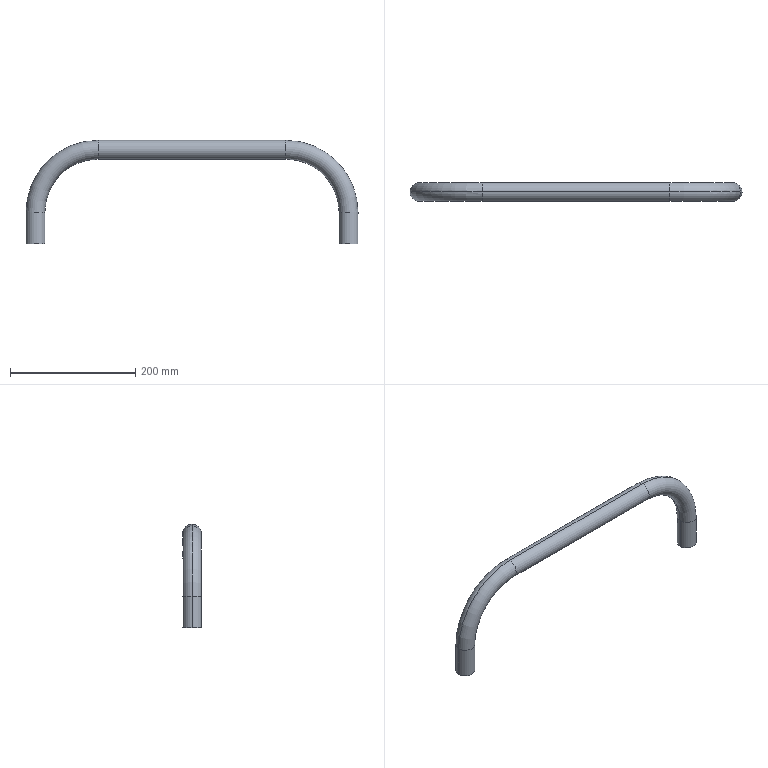Part | SolidWorks | features HoleWzd 1, Sweep 1 | 1 solid | 20 faces | box 530 x 30 x 165 mm | volume 501138 mm3 | cylinder 10 | torus 4 | cone 4 | plane 2 | commonest cylinder face diameters 30 x6 8.5 x4
STEP:
#1=CARTESIAN_POINT('',(400.,0.,15.));
#2=VERTEX_POINT('',#1);
#3=CARTESIAN_POINT('',(400.,0.,-15.));
#4=VERTEX_POINT('',#3);
#5=CARTESIAN_POINT('',(400.,0.,0.));
#6=DIRECTION('',(-1.,0.,0.));
#7=DIRECTION('',(0.,0.,1.));
#8=AXIS2_PLACEMENT_3D('',#5,#6,#7);
#9=CIRCLE('',#8,15.);
#10=EDGE_CURVE('',#2,#4,#9,.T.);
#11=ORIENTED_EDGE('',*,*,#10,.F.);
#12=CARTESIAN_POINT('',(515.,0.,-100.));
#13=VERTEX_POINT('',#12);
#14=CARTESIAN_POINT('',(400.,0.,-100.));
#15=DIRECTION('',(0.,1.,0.));
#16=DIRECTION('',(0.,0.,1.));
#17=AXIS2_PLACEMENT_3D('',#14,#15,#16);
#18=CIRCLE('',#17,115.);
#19=EDGE_CURVE('',#2,#13,#18,.T.);
#20=ORIENTED_EDGE('',*,*,#19,.T.);
#21=CARTESIAN_POINT('',(485.,0.,-100.));
#22=VERTEX_POINT('',#21);
#23=CARTESIAN_POINT('',(500.,0.,-100.));
#24=DIRECTION('',(0.,0.,1.));
#25=DIRECTION('',(1.,0.,0.));
#26=AXIS2_PLACEMENT_3D('',#23,#24,#25);
#27=CIRCLE('',#26,15.);
#28=EDGE_CURVE('',#13,#22,#27,.T.);
#29=ORIENTED_EDGE('',*,*,#28,.T.);
#30=CARTESIAN_POINT('',(400.,0.,-100.));
#31=DIRECTION('',(0.,1.,0.));
#32=DIRECTION('',(0.,0.,1.));
#33=AXIS2_PLACEMENT_3D('',#30,#31,#32);
#34=CIRCLE('',#33,85.);
#35=EDGE_CURVE('',#4,#22,#34,.T.);
#36=ORIENTED_EDGE('',*,*,#35,.F.);
#37=EDGE_LOOP('',(#11,#20,#29,#36));
#38=FACE_OUTER_BOUND('',#37,.T.);
#39=CARTESIAN_POINT('',(400.,0.,-100.));
#40=DIRECTION('',(0.,1.,0.));
#41=DIRECTION('',(0.,0.,1.));
#42=AXIS2_PLACEMENT_3D('',#39,#40,#41);
#43=TOROIDAL_SURFACE('',#42,100.,15.);
#44=ADVANCED_FACE('',(#38),#43,.T.);
#45=CARTESIAN_POINT('',(-15.,0.,-100.));
#46=VERTEX_POINT('',#45);
#47=CARTESIAN_POINT('',(15.,0.,-100.));
#48=VERTEX_POINT('',#47);
#49=CARTESIAN_POINT('',(0.,0.,-100.));
#50=DIRECTION('',(0.,0.,-1.));
#51=DIRECTION('',(-1.,0.,0.));
#52=AXIS2_PLACEMENT_3D('',#49,#50,#51);
#53=CIRCLE('',#52,15.);
#54=EDGE_CURVE('',#46,#48,#53,.T.);
#55=ORIENTED_EDGE('',*,*,#54,.F.);
#56=CARTESIAN_POINT('',(100.,0.,15.));
#57=VERTEX_POINT('',#56);
#58=CARTESIAN_POINT('',(100.,0.,-100.));
#59=DIRECTION('',(0.,1.,0.));
#60=DIRECTION('',(0.,0.,1.));
#61=AXIS2_PLACEMENT_3D('',#58,#59,#60);
#62=CIRCLE('',#61,115.);
#63=EDGE_CURVE('',#46,#57,#62,.T.);
#64=ORIENTED_EDGE('',*,*,#63,.T.);
#65=CARTESIAN_POINT('',(100.,0.,-15.));
#66=VERTEX_POINT('',#65);
#67=CARTESIAN_POINT('',(100.,0.,0.));
#68=DIRECTION('',(-1.,0.,0.));
#69=DIRECTION('',(0.,0.,1.));
#70=AXIS2_PLACEMENT_3D('',#67,#68,#69);
#71=CIRCLE('',#70,15.);
#72=EDGE_CURVE('',#57,#66,#71,.T.);
#73=ORIENTED_EDGE('',*,*,#72,.T.);
#74=CARTESIAN_POINT('',(100.,0.,-100.));
#75=DIRECTION('',(0.,1.,0.));
#76=DIRECTION('',(0.,0.,1.));
#77=AXIS2_PLACEMENT_3D('',#74,#75,#76);
#78=CIRCLE('',#77,85.);
#79=EDGE_CURVE('',#48,#66,#78,.T.);
#80=ORIENTED_EDGE('',*,*,#79,.F.);
#81=EDGE_LOOP('',(#55,#64,#73,#80));
#82=FACE_OUTER_BOUND('',#81,.T.);
#83=CARTESIAN_POINT('',(100.,0.,-100.));
#84=DIRECTION('',(0.,1.,0.));
#85=DIRECTION('',(0.,0.,1.));
#86=AXIS2_PLACEMENT_3D('',#83,#84,#85);
#87=TOROIDAL_SURFACE('',#86,100.,15.);
#88=ADVANCED_FACE('',(#82),#87,.T.);
#89=CARTESIAN_POINT('',(504.25,0.,-118.5));
#90=VERTEX_POINT('',#89);
#91=CARTESIAN_POINT('',(495.75,0.,-118.5));
#92=VERTEX_POINT('',#91);
#93=CARTESIAN_POINT('',(500.,0.,-118.5));
#94=DIRECTION('',(0.,0.,-1.));
#95=DIRECTION('',(-1.,0.,0.));
#96=AXIS2_PLACEMENT_3D('',#93,#94,#95);
#97=CIRCLE('',#96,4.25);
#98=EDGE_CURVE('',#90,#92,#97,.T.);
#99=ORIENTED_EDGE('',*,*,#98,.F.);
#100=CARTESIAN_POINT('',(504.25,0.,-150.));
#101=VERTEX_POINT('',#100);
#102=CARTESIAN_POINT('',(504.25,0.,-150.));
#103=DIRECTION('',(0.,0.,-1.));
#104=VECTOR('',#103,1000.);
#105=LINE('',#102,#104);
#106=EDGE_CURVE('',#90,#101,#105,.T.);
#107=ORIENTED_EDGE('',*,*,#106,.T.);
#108=CARTESIAN_POINT('',(495.75,0.,-150.));
#109=VERTEX_POINT('',#108);
#110=CARTESIAN_POINT('',(500.,0.,-150.));
#111=DIRECTION('',(0.,0.,-1.));
#112=DIRECTION('',(-1.,0.,0.));
#113=AXIS2_PLACEMENT_3D('',#110,#111,#112);
#114=CIRCLE('',#113,4.25);
#115=EDGE_CURVE('',#101,#109,#114,.T.);
#116=ORIENTED_EDGE('',*,*,#115,.T.);
#117=CARTESIAN_POINT('',(495.75,0.,-150.));
#118=DIRECTION('',(0.,0.,-1.));
#119=VECTOR('',#118,1000.);
#120=LINE('',#117,#119);
#121=EDGE_CURVE('',#92,#109,#120,.T.);
#122=ORIENTED_EDGE('',*,*,#121,.F.);
#123=EDGE_LOOP('',(#99,#107,#116,#122));
#124=FACE_OUTER_BOUND('',#123,.T.);
#125=CARTESIAN_POINT('',(500.,0.,-150.));
#126=DIRECTION('',(0.,0.,-1.));
#127=DIRECTION('',(-1.,0.,0.));
#128=AXIS2_PLACEMENT_3D('',#125,#126,#127);
#129=CYLINDRICAL_SURFACE('',#128,4.25);
#130=ADVANCED_FACE('',(#124),#129,.F.);
#131=CARTESIAN_POINT('',(500.,0.,-115.946));
#132=VERTEX_POINT('',#131);
#133=CARTESIAN_POINT('',(495.75,0.,-118.5));
#134=DIRECTION('',(-0.8572,0.,-0.515));
#135=VECTOR('',#134,1000.);
#136=LINE('',#133,#135);
#137=EDGE_CURVE('',#132,#92,#136,.T.);
#138=ORIENTED_EDGE('',*,*,#137,.F.);
#139=CARTESIAN_POINT('',(504.25,0.,-118.5));
#140=DIRECTION('',(0.8572,0.,-0.515));
#141=VECTOR('',#140,1000.);
#142=LINE('',#139,#141);
#143=EDGE_CURVE('',#132,#90,#142,.T.);
#144=ORIENTED_EDGE('',*,*,#143,.T.);
#145=ORIENTED_EDGE('',*,*,#98,.T.);
#146=EDGE_LOOP('',(#138,#144,#145));
#147=FACE_OUTER_BOUND('',#146,.T.);
#148=CARTESIAN_POINT('',(500.,0.,-118.5));
#149=DIRECTION('',(0.,0.,-1.));
#150=DIRECTION('',(-1.,0.,0.));
#151=AXIS2_PLACEMENT_3D('',#148,#149,#150);
#152=CONICAL_SURFACE('',#151,4.25,1.03);
#153=ADVANCED_FACE('',(#147),#152,.F.);
#154=CARTESIAN_POINT('',(4.25,0.,-118.5));
#155=VERTEX_POINT('',#154);
#156=CARTESIAN_POINT('',(-4.25,0.,-118.5));
#157=VERTEX_POINT('',#156);
#158=CARTESIAN_POINT('',(0.,0.,-118.5));
#159=DIRECTION('',(0.,0.,-1.));
#160=DIRECTION('',(-1.,0.,0.));
#161=AXIS2_PLACEMENT_3D('',#158,#159,#160);
#162=CIRCLE('',#161,4.25);
#163=EDGE_CURVE('',#155,#157,#162,.T.);
#164=ORIENTED_EDGE('',*,*,#163,.F.);
#165=CARTESIAN_POINT('',(4.25,0.,-150.));
#166=VERTEX_POINT('',#165);
#167=CARTESIAN_POINT('',(4.25,0.,-150.));
#168=DIRECTION('',(0.,0.,-1.));
#169=VECTOR('',#168,1000.);
#170=LINE('',#167,#169);
#171=EDGE_CURVE('',#155,#166,#170,.T.);
#172=ORIENTED_EDGE('',*,*,#171,.T.);
#173=CARTESIAN_POINT('',(-4.25,0.,-150.));
#174=VERTEX_POINT('',#173);
#175=CARTESIAN_POINT('',(0.,0.,-150.));
#176=DIRECTION('',(0.,0.,-1.));
#177=DIRECTION('',(-1.,0.,0.));
#178=AXIS2_PLACEMENT_3D('',#175,#176,#177);
#179=CIRCLE('',#178,4.25);
#180=EDGE_CURVE('',#166,#174,#179,.T.);
#181=ORIENTED_EDGE('',*,*,#180,.T.);
#182=CARTESIAN_POINT('',(-4.25,0.,-150.));
#183=DIRECTION('',(0.,0.,-1.));
#184=VECTOR('',#183,1000.);
#185=LINE('',#182,#184);
#186=EDGE_CURVE('',#157,#174,#185,.T.);
#187=ORIENTED_EDGE('',*,*,#186,.F.);
#188=EDGE_LOOP('',(#164,#172,#181,#187));
#189=FACE_OUTER_BOUND('',#188,.T.);
#190=CARTESIAN_POINT('',(0.,0.,-150.));
#191=DIRECTION('',(0.,0.,-1.));
#192=DIRECTION('',(-1.,0.,0.));
#193=AXIS2_PLACEMENT_3D('',#190,#191,#192);
#194=CYLINDRICAL_SURFACE('',#193,4.25);
#195=ADVANCED_FACE('',(#189),#194,.F.);
#196=CARTESIAN_POINT('',(0.,0.,-115.946));
#197=VERTEX_POINT('',#196);
#198=CARTESIAN_POINT('',(-4.25,0.,-118.5));
#199=DIRECTION('',(-0.8572,0.,-0.515));
#200=VECTOR('',#199,1000.);
#201=LINE('',#198,#200);
#202=EDGE_CURVE('',#197,#157,#201,.T.);
#203=ORIENTED_EDGE('',*,*,#202,.F.);
#204=CARTESIAN_POINT('',(4.25,0.,-118.5));
#205=DIRECTION('',(0.8572,0.,-0.515));
#206=VECTOR('',#205,1000.);
#207=LINE('',#204,#206);
#208=EDGE_CURVE('',#197,#155,#207,.T.);
#209=ORIENTED_EDGE('',*,*,#208,.T.);
#210=ORIENTED_EDGE('',*,*,#163,.T.);
#211=EDGE_LOOP('',(#203,#209,#210));
#212=FACE_OUTER_BOUND('',#211,.T.);
#213=CARTESIAN_POINT('',(0.,0.,-118.5));
#214=DIRECTION('',(0.,0.,-1.));
#215=DIRECTION('',(-1.,0.,0.));
#216=AXIS2_PLACEMENT_3D('',#213,#214,#215);
#217=CONICAL_SURFACE('',#216,4.25,1.03);
#218=ADVANCED_FACE('',(#212),#217,.F.);
#219=ORIENTED_EDGE('',*,*,#28,.F.);
#220=CARTESIAN_POINT('',(515.,0.,-150.));
#221=VERTEX_POINT('',#220);
#222=CARTESIAN_POINT('',(515.,0.,-100.));
#223=DIRECTION('',(0.,0.,-1.));
#224=VECTOR('',#223,1000.);
#225=LINE('',#222,#224);
#226=EDGE_CURVE('',#13,#221,#225,.T.);
#227=ORIENTED_EDGE('',*,*,#226,.T.);
#228=CARTESIAN_POINT('',(485.,0.,-150.));
#229=VERTEX_POINT('',#228);
#230=CARTESIAN_POINT('',(500.,0.,-150.));
#231=DIRECTION('',(0.,0.,1.));
#232=DIRECTION('',(1.,0.,0.));
#233=AXIS2_PLACEMENT_3D('',#230,#231,#232);
#234=CIRCLE('',#233,15.);
#235=EDGE_CURVE('',#221,#229,#234,.T.);
#236=ORIENTED_EDGE('',*,*,#235,.T.);
#237=CARTESIAN_POINT('',(485.,0.,-100.));
#238=DIRECTION('',(0.,0.,-1.));
#239=VECTOR('',#238,1000.);
#240=LINE('',#237,#239);
#241=EDGE_CURVE('',#22,#229,#240,.T.);
#242=ORIENTED_EDGE('',*,*,#241,.F.);
#243=EDGE_LOOP('',(#219,#227,#236,#242));
#244=FACE_OUTER_BOUND('',#243,.T.);
#245=CARTESIAN_POINT('',(500.,0.,-100.));
#246=DIRECTION('',(0.,0.,-1.));
#247=DIRECTION('',(-1.,0.,0.));
#248=AXIS2_PLACEMENT_3D('',#245,#246,#247);
#249=CYLINDRICAL_SURFACE('',#248,15.);
#250=ADVANCED_FACE('',(#244),#249,.T.);
#251=ORIENTED_EDGE('',*,*,#72,.F.);
#252=CARTESIAN_POINT('',(100.,0.,15.));
#253=DIRECTION('',(1.,0.,0.));
#254=VECTOR('',#253,1000.);
#255=LINE('',#252,#254);
#256=EDGE_CURVE('',#57,#2,#255,.T.);
#257=ORIENTED_EDGE('',*,*,#256,.T.);
#258=ORIENTED_EDGE('',*,*,#10,.T.);
#259=CARTESIAN_POINT('',(100.,0.,-15.));
#260=DIRECTION('',(1.,0.,0.));
#261=VECTOR('',#260,1000.);
#262=LINE('',#259,#261);
#263=EDGE_CURVE('',#66,#4,#262,.T.);
#264=ORIENTED_EDGE('',*,*,#263,.F.);
#265=EDGE_LOOP('',(#251,#257,#258,#264));
#266=FACE_OUTER_BOUND('',#265,.T.);
#267=CARTESIAN_POINT('',(100.,0.,0.));
#268=DIRECTION('',(1.,0.,0.));
#269=DIRECTION('',(0.,0.,-1.));
#270=AXIS2_PLACEMENT_3D('',#267,#268,#269);
#271=CYLINDRICAL_SURFACE('',#270,15.);
#272=ADVANCED_FACE('',(#266),#271,.T.);
#273=CARTESIAN_POINT('',(-15.,0.,-150.));
#274=VERTEX_POINT('',#273);
#275=CARTESIAN_POINT('',(15.,0.,-150.));
#276=VERTEX_POINT('',#275);
#277=CARTESIAN_POINT('',(0.,0.,-150.));
#278=DIRECTION('',(0.,0.,-1.));
#279=DIRECTION('',(-1.,0.,0.));
#280=AXIS2_PLACEMENT_3D('',#277,#278,#279);
#281=CIRCLE('',#280,15.);
#282=EDGE_CURVE('',#274,#276,#281,.T.);
#283=ORIENTED_EDGE('',*,*,#282,.F.);
#284=CARTESIAN_POINT('',(-15.,0.,-150.));
#285=DIRECTION('',(0.,0.,1.));
#286=VECTOR('',#285,1000.);
#287=LINE('',#284,#286);
#288=EDGE_CURVE('',#274,#46,#287,.T.);
#289=ORIENTED_EDGE('',*,*,#288,.T.);
#290=ORIENTED_EDGE('',*,*,#54,.T.);
#291=CARTESIAN_POINT('',(15.,0.,-150.));
#292=DIRECTION('',(0.,0.,1.));
#293=VECTOR('',#292,1000.);
#294=LINE('',#291,#293);
#295=EDGE_CURVE('',#276,#48,#294,.T.);
#296=ORIENTED_EDGE('',*,*,#295,.F.);
#297=EDGE_LOOP('',(#283,#289,#290,#296));
#298=FACE_OUTER_BOUND('',#297,.T.);
#299=CARTESIAN_POINT('',(0.,0.,-150.));
#300=DIRECTION('',(0.,0.,1.));
#301=DIRECTION('',(1.,0.,0.));
#302=AXIS2_PLACEMENT_3D('',#299,#300,#301);
#303=CYLINDRICAL_SURFACE('',#302,15.);
#304=ADVANCED_FACE('',(#298),#303,.T.);
#305=CARTESIAN_POINT('',(500.,0.,-150.));
#306=DIRECTION('',(0.,0.,1.));
#307=DIRECTION('',(1.,0.,0.));
#308=AXIS2_PLACEMENT_3D('',#305,#306,#307);
#309=CIRCLE('',#308,15.);
#310=EDGE_CURVE('',#229,#221,#309,.T.);
#311=ORIENTED_EDGE('',*,*,#310,.F.);
#312=ORIENTED_EDGE('',*,*,#235,.F.);
#313=EDGE_LOOP('',(#311,#312));
#314=FACE_OUTER_BOUND('',#313,.T.);
#315=CARTESIAN_POINT('',(500.,0.,-150.));
#316=DIRECTION('',(0.,0.,-1.));
#317=DIRECTION('',(-1.,0.,0.));
#318=AXIS2_PLACEMENT_3D('',#315,#316,#317);
#319=CIRCLE('',#318,4.25);
#320=EDGE_CURVE('',#109,#101,#319,.T.);
#321=ORIENTED_EDGE('',*,*,#320,.F.);
#322=ORIENTED_EDGE('',*,*,#115,.F.);
#323=EDGE_LOOP('',(#321,#322));
#324=FACE_BOUND('',#323,.T.);
#325=CARTESIAN_POINT('',(500.,0.,-150.));
#326=DIRECTION('',(0.,0.,1.));
#327=DIRECTION('',(1.,0.,0.));
#328=AXIS2_PLACEMENT_3D('',#325,#326,#327);
#329=PLANE('',#328);
#330=ADVANCED_FACE('',(#314,#324),#329,.F.);
#331=ORIENTED_EDGE('',*,*,#226,.F.);
#332=CARTESIAN_POINT('',(500.,0.,-100.));
#333=DIRECTION('',(0.,0.,1.));
#334=DIRECTION('',(1.,0.,0.));
#335=AXIS2_PLACEMENT_3D('',#332,#333,#334);
#336=CIRCLE('',#335,15.);
#337=EDGE_CURVE('',#22,#13,#336,.T.);
#338=ORIENTED_EDGE('',*,*,#337,.F.);
#339=ORIENTED_EDGE('',*,*,#241,.T.);
#340=ORIENTED_EDGE('',*,*,#310,.T.);
#341=EDGE_LOOP('',(#331,#338,#339,#340));
#342=FACE_OUTER_BOUND('',#341,.T.);
#343=CARTESIAN_POINT('',(500.,0.,-100.));
#344=DIRECTION('',(0.,0.,-1.));
#345=DIRECTION('',(-1.,0.,0.));
#346=AXIS2_PLACEMENT_3D('',#343,#344,#345);
#347=CYLINDRICAL_SURFACE('',#346,15.);
#348=ADVANCED_FACE('',(#342),#347,.T.);
#349=ORIENTED_EDGE('',*,*,#19,.F.);
#350=CARTESIAN_POINT('',(400.,0.,0.));
#351=DIRECTION('',(-1.,0.,0.));
#352=DIRECTION('',(0.,0.,1.));
#353=AXIS2_PLACEMENT_3D('',#350,#351,#352);
#354=CIRCLE('',#353,15.);
#355=EDGE_CURVE('',#4,#2,#354,.T.);
#356=ORIENTED_EDGE('',*,*,#355,.F.);
#357=ORIENTED_EDGE('',*,*,#35,.T.);
#358=ORIENTED_EDGE('',*,*,#337,.T.);
#359=EDGE_LOOP('',(#349,#356,#357,#358));
#360=FACE_OUTER_BOUND('',#359,.T.);
#361=CARTESIAN_POINT('',(400.,0.,-100.));
#362=DIRECTION('',(0.,1.,0.));
#363=DIRECTION('',(0.,0.,1.));
#364=AXIS2_PLACEMENT_3D('',#361,#362,#363);
#365=TOROIDAL_SURFACE('',#364,100.,15.);
#366=ADVANCED_FACE('',(#360),#365,.T.);
#367=ORIENTED_EDGE('',*,*,#256,.F.);
#368=CARTESIAN_POINT('',(100.,0.,0.));
#369=DIRECTION('',(-1.,0.,0.));
#370=DIRECTION('',(0.,0.,1.));
#371=AXIS2_PLACEMENT_3D('',#368,#369,#370);
#372=CIRCLE('',#371,15.);
#373=EDGE_CURVE('',#66,#57,#372,.T.);
#374=ORIENTED_EDGE('',*,*,#373,.F.);
#375=ORIENTED_EDGE('',*,*,#263,.T.);
#376=ORIENTED_EDGE('',*,*,#355,.T.);
#377=EDGE_LOOP('',(#367,#374,#375,#376));
#378=FACE_OUTER_BOUND('',#377,.T.);
#379=CARTESIAN_POINT('',(100.,0.,0.));
#380=DIRECTION('',(1.,0.,0.));
#381=DIRECTION('',(0.,0.,-1.));
#382=AXIS2_PLACEMENT_3D('',#379,#380,#381);
#383=CYLINDRICAL_SURFACE('',#382,15.);
#384=ADVANCED_FACE('',(#378),#383,.T.);
#385=ORIENTED_EDGE('',*,*,#63,.F.);
#386=CARTESIAN_POINT('',(0.,0.,-100.));
#387=DIRECTION('',(0.,0.,-1.));
#388=DIRECTION('',(-1.,0.,0.));
#389=AXIS2_PLACEMENT_3D('',#386,#387,#388);
#390=CIRCLE('',#389,15.);
#391=EDGE_CURVE('',#48,#46,#390,.T.);
#392=ORIENTED_EDGE('',*,*,#391,.F.);
#393=ORIENTED_EDGE('',*,*,#79,.T.);
#394=ORIENTED_EDGE('',*,*,#373,.T.);
#395=EDGE_LOOP('',(#385,#392,#393,#394));
#396=FACE_OUTER_BOUND('',#395,.T.);
#397=CARTESIAN_POINT('',(100.,0.,-100.));
#398=DIRECTION('',(0.,1.,0.));
#399=DIRECTION('',(0.,0.,1.));
#400=AXIS2_PLACEMENT_3D('',#397,#398,#399);
#401=TOROIDAL_SURFACE('',#400,100.,15.);
#402=ADVANCED_FACE('',(#396),#401,.T.);
#403=ORIENTED_EDGE('',*,*,#288,.F.);
#404=CARTESIAN_POINT('',(0.,0.,-150.));
#405=DIRECTION('',(0.,0.,-1.));
#406=DIRECTION('',(-1.,0.,0.));
#407=AXIS2_PLACEMENT_3D('',#404,#405,#406);
#408=CIRCLE('',#407,15.);
#409=EDGE_CURVE('',#276,#274,#408,.T.);
#410=ORIENTED_EDGE('',*,*,#409,.F.);
#411=ORIENTED_EDGE('',*,*,#295,.T.);
#412=ORIENTED_EDGE('',*,*,#391,.T.);
#413=EDGE_LOOP('',(#403,#410,#411,#412));
#414=FACE_OUTER_BOUND('',#413,.T.);
#415=CARTESIAN_POINT('',(0.,0.,-150.));
#416=DIRECTION('',(0.,0.,1.));
#417=DIRECTION('',(1.,0.,0.));
#418=AXIS2_PLACEMENT_3D('',#415,#416,#417);
#419=CYLINDRICAL_SURFACE('',#418,15.);
#420=ADVANCED_FACE('',(#414),#419,.T.);
#421=CARTESIAN_POINT('',(0.,0.,-150.));
#422=DIRECTION('',(0.,0.,-1.));
#423=DIRECTION('',(-1.,0.,0.));
#424=AXIS2_PLACEMENT_3D('',#421,#422,#423);
#425=CIRCLE('',#424,4.25);
#426=EDGE_CURVE('',#174,#166,#425,.T.);
#427=ORIENTED_EDGE('',*,*,#426,.F.);
#428=ORIENTED_EDGE('',*,*,#180,.F.);
#429=EDGE_LOOP('',(#427,#428));
#430=FACE_BOUND('',#429,.T.);
#431=ORIENTED_EDGE('',*,*,#409,.T.);
#432=ORIENTED_EDGE('',*,*,#282,.T.);
#433=EDGE_LOOP('',(#431,#432));
#434=FACE_OUTER_BOUND('',#433,.T.);
#435=CARTESIAN_POINT('',(0.,0.,-150.));
#436=DIRECTION('',(0.,0.,-1.));
#437=DIRECTION('',(-1.,0.,0.));
#438=AXIS2_PLACEMENT_3D('',#435,#436,#437);
#439=PLANE('',#438);
#440=ADVANCED_FACE('',(#430,#434),#439,.T.);
#441=ORIENTED_EDGE('',*,*,#208,.F.);
#442=ORIENTED_EDGE('',*,*,#202,.T.);
#443=CARTESIAN_POINT('',(0.,0.,-118.5));
#444=DIRECTION('',(0.,0.,-1.));
#445=DIRECTION('',(-1.,0.,0.));
#446=AXIS2_PLACEMENT_3D('',#443,#444,#445);
#447=CIRCLE('',#446,4.25);
#448=EDGE_CURVE('',#157,#155,#447,.T.);
#449=ORIENTED_EDGE('',*,*,#448,.T.);
#450=EDGE_LOOP('',(#441,#442,#449));
#451=FACE_OUTER_BOUND('',#450,.T.);
#452=CARTESIAN_POINT('',(0.,0.,-118.5));
#453=DIRECTION('',(0.,0.,-1.));
#454=DIRECTION('',(-1.,0.,0.));
#455=AXIS2_PLACEMENT_3D('',#452,#453,#454);
#456=CONICAL_SURFACE('',#455,4.25,1.03);
#457=ADVANCED_FACE('',(#451),#456,.F.);
#458=ORIENTED_EDGE('',*,*,#171,.F.);
#459=ORIENTED_EDGE('',*,*,#448,.F.);
#460=ORIENTED_EDGE('',*,*,#186,.T.);
#461=ORIENTED_EDGE('',*,*,#426,.T.);
#462=EDGE_LOOP('',(#458,#459,#460,#461));
#463=FACE_OUTER_BOUND('',#462,.T.);
#464=CARTESIAN_POINT('',(0.,0.,-150.));
#465=DIRECTION('',(0.,0.,-1.));
#466=DIRECTION('',(-1.,0.,0.));
#467=AXIS2_PLACEMENT_3D('',#464,#465,#466);
#468=CYLINDRICAL_SURFACE('',#467,4.25);
#469=ADVANCED_FACE('',(#463),#468,.F.);
#470=ORIENTED_EDGE('',*,*,#143,.F.);
#471=ORIENTED_EDGE('',*,*,#137,.T.);
#472=CARTESIAN_POINT('',(500.,0.,-118.5));
#473=DIRECTION('',(0.,0.,-1.));
#474=DIRECTION('',(-1.,0.,0.));
#475=AXIS2_PLACEMENT_3D('',#472,#473,#474);
#476=CIRCLE('',#475,4.25);
#477=EDGE_CURVE('',#92,#90,#476,.T.);
#478=ORIENTED_EDGE('',*,*,#477,.T.);
#479=EDGE_LOOP('',(#470,#471,#478));
#480=FACE_OUTER_BOUND('',#479,.T.);
#481=CARTESIAN_POINT('',(500.,0.,-118.5));
#482=DIRECTION('',(0.,0.,-1.));
#483=DIRECTION('',(-1.,0.,0.));
#484=AXIS2_PLACEMENT_3D('',#481,#482,#483);
#485=CONICAL_SURFACE('',#484,4.25,1.03);
#486=ADVANCED_FACE('',(#480),#485,.F.);
#487=ORIENTED_EDGE('',*,*,#106,.F.);
#488=ORIENTED_EDGE('',*,*,#477,.F.);
#489=ORIENTED_EDGE('',*,*,#121,.T.);
#490=ORIENTED_EDGE('',*,*,#320,.T.);
#491=EDGE_LOOP('',(#487,#488,#489,#490));
#492=FACE_OUTER_BOUND('',#491,.T.);
#493=CARTESIAN_POINT('',(500.,0.,-150.));
#494=DIRECTION('',(0.,0.,-1.));
#495=DIRECTION('',(-1.,0.,0.));
#496=AXIS2_PLACEMENT_3D('',#493,#494,#495);
#497=CYLINDRICAL_SURFACE('',#496,4.25);
#498=ADVANCED_FACE('',(#492),#497,.F.);
#499=CLOSED_SHELL('',(#44,#88,#130,#153,#195,#218,#250,#272,#304,#330,#348,#366,#384,#402,#420,#440,#457,#469,#486,#498));
#500=MANIFOLD_SOLID_BREP('',#499);
#501=CARTESIAN_POINT('',(0.,0.,0.));
#502=DIRECTION('',(0.,0.,1.));
#503=DIRECTION('',(1.,0.,0.));
#504=AXIS2_PLACEMENT_3D('',#501,#502,#503);
#505=(LENGTH_UNIT()NAMED_UNIT(*)SI_UNIT(.MILLI.,.METRE.));
#506=UNCERTAINTY_MEASURE_WITH_UNIT(LENGTH_MEASURE(0.00001),#505,'','');
#507=(NAMED_UNIT(*)PLANE_ANGLE_UNIT()SI_UNIT($,.RADIAN.));
#508=(NAMED_UNIT(*)SI_UNIT($,.STERADIAN.)SOLID_ANGLE_UNIT());
#509=(GEOMETRIC_REPRESENTATION_CONTEXT(3)GLOBAL_UNCERTAINTY_ASSIGNED_CONTEXT((#506))GLOBAL_UNIT_ASSIGNED_CONTEXT((#505,#507,#508))REPRESENTATION_CONTEXT('',''));
#510=ADVANCED_BREP_SHAPE_REPRESENTATION('',(#500,#504),#509);